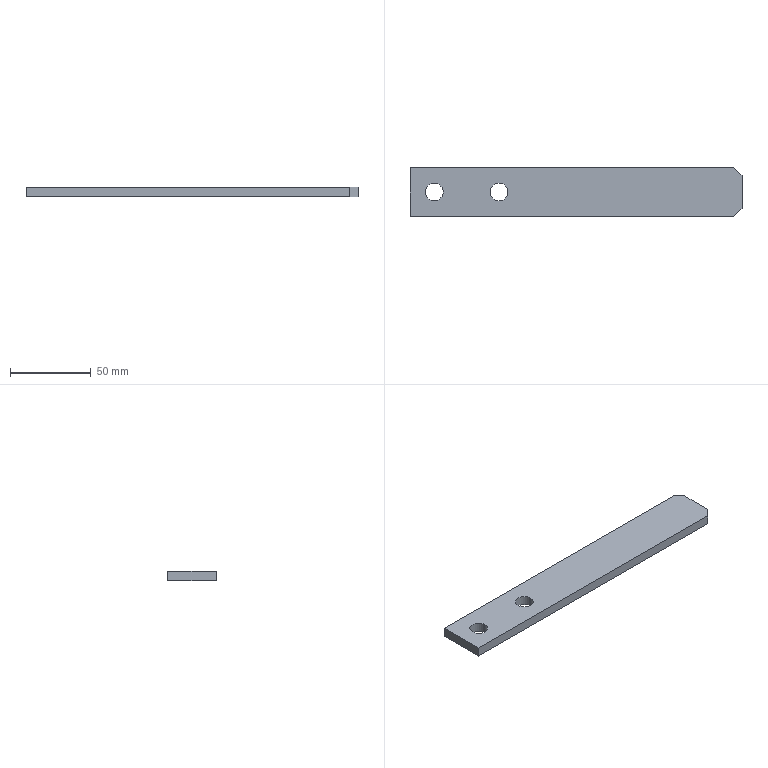Part | SolidWorks | features Extrusion 1 | 1 solid | 12 faces | box 205 x 30 x 6 mm | volume 35610 mm3 | plane 8 | cylinder 4 | commonest cylinder face diameters 11 x4
STEP:
#1=CARTESIAN_POINT('',(-53.,0.,-3.));
#2=VERTEX_POINT('',#1);
#3=CARTESIAN_POINT('',(-42.,0.,-3.));
#4=VERTEX_POINT('',#3);
#5=CARTESIAN_POINT('',(-47.5,0.,-3.));
#6=DIRECTION('',(0.,0.,1.));
#7=DIRECTION('',(-1.,0.,0.));
#8=AXIS2_PLACEMENT_3D('',#5,#6,#7);
#9=CIRCLE('',#8,5.5);
#10=EDGE_CURVE('',#2,#4,#9,.T.);
#11=ORIENTED_EDGE('',*,*,#10,.F.);
#12=CARTESIAN_POINT('',(-53.,0.,3.));
#13=VERTEX_POINT('',#12);
#14=CARTESIAN_POINT('',(-53.,0.,-3.));
#15=DIRECTION('',(0.,0.,1.));
#16=VECTOR('',#15,1000.);
#17=LINE('',#14,#16);
#18=EDGE_CURVE('',#2,#13,#17,.T.);
#19=ORIENTED_EDGE('',*,*,#18,.T.);
#20=CARTESIAN_POINT('',(-42.,0.,3.));
#21=VERTEX_POINT('',#20);
#22=CARTESIAN_POINT('',(-47.5,0.,3.));
#23=DIRECTION('',(0.,0.,1.));
#24=DIRECTION('',(-1.,0.,0.));
#25=AXIS2_PLACEMENT_3D('',#22,#23,#24);
#26=CIRCLE('',#25,5.5);
#27=EDGE_CURVE('',#13,#21,#26,.T.);
#28=ORIENTED_EDGE('',*,*,#27,.T.);
#29=CARTESIAN_POINT('',(-42.,0.,-3.));
#30=DIRECTION('',(0.,0.,1.));
#31=VECTOR('',#30,1000.);
#32=LINE('',#29,#31);
#33=EDGE_CURVE('',#4,#21,#32,.T.);
#34=ORIENTED_EDGE('',*,*,#33,.F.);
#35=EDGE_LOOP('',(#11,#19,#28,#34));
#36=FACE_OUTER_BOUND('',#35,.T.);
#37=CARTESIAN_POINT('',(-47.5,0.,-3.));
#38=DIRECTION('',(0.,0.,1.));
#39=DIRECTION('',(1.,0.,0.));
#40=AXIS2_PLACEMENT_3D('',#37,#38,#39);
#41=CYLINDRICAL_SURFACE('',#40,5.5);
#42=ADVANCED_FACE('',(#36),#41,.F.);
#43=CARTESIAN_POINT('',(-93.,0.,-3.));
#44=VERTEX_POINT('',#43);
#45=CARTESIAN_POINT('',(-82.,0.,-3.));
#46=VERTEX_POINT('',#45);
#47=CARTESIAN_POINT('',(-87.5,0.,-3.));
#48=DIRECTION('',(0.,0.,1.));
#49=DIRECTION('',(-1.,0.,0.));
#50=AXIS2_PLACEMENT_3D('',#47,#48,#49);
#51=CIRCLE('',#50,5.5);
#52=EDGE_CURVE('',#44,#46,#51,.T.);
#53=ORIENTED_EDGE('',*,*,#52,.F.);
#54=CARTESIAN_POINT('',(-93.,0.,3.));
#55=VERTEX_POINT('',#54);
#56=CARTESIAN_POINT('',(-93.,0.,-3.));
#57=DIRECTION('',(0.,0.,1.));
#58=VECTOR('',#57,1000.);
#59=LINE('',#56,#58);
#60=EDGE_CURVE('',#44,#55,#59,.T.);
#61=ORIENTED_EDGE('',*,*,#60,.T.);
#62=CARTESIAN_POINT('',(-82.,0.,3.));
#63=VERTEX_POINT('',#62);
#64=CARTESIAN_POINT('',(-87.5,0.,3.));
#65=DIRECTION('',(0.,0.,1.));
#66=DIRECTION('',(-1.,0.,0.));
#67=AXIS2_PLACEMENT_3D('',#64,#65,#66);
#68=CIRCLE('',#67,5.5);
#69=EDGE_CURVE('',#55,#63,#68,.T.);
#70=ORIENTED_EDGE('',*,*,#69,.T.);
#71=CARTESIAN_POINT('',(-82.,0.,-3.));
#72=DIRECTION('',(0.,0.,1.));
#73=VECTOR('',#72,1000.);
#74=LINE('',#71,#73);
#75=EDGE_CURVE('',#46,#63,#74,.T.);
#76=ORIENTED_EDGE('',*,*,#75,.F.);
#77=EDGE_LOOP('',(#53,#61,#70,#76));
#78=FACE_OUTER_BOUND('',#77,.T.);
#79=CARTESIAN_POINT('',(-87.5,0.,-3.));
#80=DIRECTION('',(0.,0.,1.));
#81=DIRECTION('',(1.,0.,0.));
#82=AXIS2_PLACEMENT_3D('',#79,#80,#81);
#83=CYLINDRICAL_SURFACE('',#82,5.5);
#84=ADVANCED_FACE('',(#78),#83,.F.);
#85=CARTESIAN_POINT('',(97.5,-15.,3.));
#86=VERTEX_POINT('',#85);
#87=CARTESIAN_POINT('',(102.5,-10.,3.));
#88=VERTEX_POINT('',#87);
#89=CARTESIAN_POINT('',(97.5,-15.,3.));
#90=DIRECTION('',(0.7071,0.7071,0.));
#91=VECTOR('',#90,1000.);
#92=LINE('',#89,#91);
#93=EDGE_CURVE('',#86,#88,#92,.T.);
#94=ORIENTED_EDGE('',*,*,#93,.F.);
#95=CARTESIAN_POINT('',(97.5,-15.,-3.));
#96=VERTEX_POINT('',#95);
#97=CARTESIAN_POINT('',(97.5,-15.,-3.));
#98=DIRECTION('',(0.,0.,1.));
#99=VECTOR('',#98,1000.);
#100=LINE('',#97,#99);
#101=EDGE_CURVE('',#96,#86,#100,.T.);
#102=ORIENTED_EDGE('',*,*,#101,.F.);
#103=CARTESIAN_POINT('',(102.5,-10.,-3.));
#104=VERTEX_POINT('',#103);
#105=CARTESIAN_POINT('',(97.5,-15.,-3.));
#106=DIRECTION('',(0.7071,0.7071,0.));
#107=VECTOR('',#106,1000.);
#108=LINE('',#105,#107);
#109=EDGE_CURVE('',#96,#104,#108,.T.);
#110=ORIENTED_EDGE('',*,*,#109,.T.);
#111=CARTESIAN_POINT('',(102.5,-10.,-3.));
#112=DIRECTION('',(0.,0.,1.));
#113=VECTOR('',#112,1000.);
#114=LINE('',#111,#113);
#115=EDGE_CURVE('',#104,#88,#114,.T.);
#116=ORIENTED_EDGE('',*,*,#115,.T.);
#117=EDGE_LOOP('',(#94,#102,#110,#116));
#118=FACE_OUTER_BOUND('',#117,.T.);
#119=CARTESIAN_POINT('',(97.5,-15.,-3.));
#120=DIRECTION('',(0.7071,-0.7071,0.));
#121=DIRECTION('',(0.7071,0.7071,0.));
#122=AXIS2_PLACEMENT_3D('',#119,#120,#121);
#123=PLANE('',#122);
#124=ADVANCED_FACE('',(#118),#123,.T.);
#125=CARTESIAN_POINT('',(-102.5,-15.,3.));
#126=VERTEX_POINT('',#125);
#127=CARTESIAN_POINT('',(-102.5,-15.,3.));
#128=DIRECTION('',(1.,0.,0.));
#129=VECTOR('',#128,1000.);
#130=LINE('',#127,#129);
#131=EDGE_CURVE('',#126,#86,#130,.T.);
#132=ORIENTED_EDGE('',*,*,#131,.F.);
#133=CARTESIAN_POINT('',(-102.5,-15.,-3.));
#134=VERTEX_POINT('',#133);
#135=CARTESIAN_POINT('',(-102.5,-15.,-3.));
#136=DIRECTION('',(0.,0.,1.));
#137=VECTOR('',#136,1000.);
#138=LINE('',#135,#137);
#139=EDGE_CURVE('',#134,#126,#138,.T.);
#140=ORIENTED_EDGE('',*,*,#139,.F.);
#141=CARTESIAN_POINT('',(-102.5,-15.,-3.));
#142=DIRECTION('',(1.,0.,0.));
#143=VECTOR('',#142,1000.);
#144=LINE('',#141,#143);
#145=EDGE_CURVE('',#134,#96,#144,.T.);
#146=ORIENTED_EDGE('',*,*,#145,.T.);
#147=ORIENTED_EDGE('',*,*,#101,.T.);
#148=EDGE_LOOP('',(#132,#140,#146,#147));
#149=FACE_OUTER_BOUND('',#148,.T.);
#150=CARTESIAN_POINT('',(-102.5,-15.,-3.));
#151=DIRECTION('',(0.,-1.,0.));
#152=DIRECTION('',(0.,0.,-1.));
#153=AXIS2_PLACEMENT_3D('',#150,#151,#152);
#154=PLANE('',#153);
#155=ADVANCED_FACE('',(#149),#154,.T.);
#156=CARTESIAN_POINT('',(-102.5,15.,3.));
#157=VERTEX_POINT('',#156);
#158=CARTESIAN_POINT('',(-102.5,15.,3.));
#159=DIRECTION('',(0.,-1.,0.));
#160=VECTOR('',#159,1000.);
#161=LINE('',#158,#160);
#162=EDGE_CURVE('',#157,#126,#161,.T.);
#163=ORIENTED_EDGE('',*,*,#162,.F.);
#164=CARTESIAN_POINT('',(-102.5,15.,-3.));
#165=VERTEX_POINT('',#164);
#166=CARTESIAN_POINT('',(-102.5,15.,-3.));
#167=DIRECTION('',(0.,0.,1.));
#168=VECTOR('',#167,1000.);
#169=LINE('',#166,#168);
#170=EDGE_CURVE('',#165,#157,#169,.T.);
#171=ORIENTED_EDGE('',*,*,#170,.F.);
#172=CARTESIAN_POINT('',(-102.5,15.,-3.));
#173=DIRECTION('',(0.,-1.,0.));
#174=VECTOR('',#173,1000.);
#175=LINE('',#172,#174);
#176=EDGE_CURVE('',#165,#134,#175,.T.);
#177=ORIENTED_EDGE('',*,*,#176,.T.);
#178=ORIENTED_EDGE('',*,*,#139,.T.);
#179=EDGE_LOOP('',(#163,#171,#177,#178));
#180=FACE_OUTER_BOUND('',#179,.T.);
#181=CARTESIAN_POINT('',(-102.5,15.,-3.));
#182=DIRECTION('',(-1.,0.,0.));
#183=DIRECTION('',(0.,0.,1.));
#184=AXIS2_PLACEMENT_3D('',#181,#182,#183);
#185=PLANE('',#184);
#186=ADVANCED_FACE('',(#180),#185,.T.);
#187=CARTESIAN_POINT('',(97.5,15.,3.));
#188=VERTEX_POINT('',#187);
#189=CARTESIAN_POINT('',(97.5,15.,3.));
#190=DIRECTION('',(-1.,0.,0.));
#191=VECTOR('',#190,1000.);
#192=LINE('',#189,#191);
#193=EDGE_CURVE('',#188,#157,#192,.T.);
#194=ORIENTED_EDGE('',*,*,#193,.F.);
#195=CARTESIAN_POINT('',(97.5,15.,-3.));
#196=VERTEX_POINT('',#195);
#197=CARTESIAN_POINT('',(97.5,15.,-3.));
#198=DIRECTION('',(0.,0.,1.));
#199=VECTOR('',#198,1000.);
#200=LINE('',#197,#199);
#201=EDGE_CURVE('',#196,#188,#200,.T.);
#202=ORIENTED_EDGE('',*,*,#201,.F.);
#203=CARTESIAN_POINT('',(97.5,15.,-3.));
#204=DIRECTION('',(-1.,0.,0.));
#205=VECTOR('',#204,1000.);
#206=LINE('',#203,#205);
#207=EDGE_CURVE('',#196,#165,#206,.T.);
#208=ORIENTED_EDGE('',*,*,#207,.T.);
#209=ORIENTED_EDGE('',*,*,#170,.T.);
#210=EDGE_LOOP('',(#194,#202,#208,#209));
#211=FACE_OUTER_BOUND('',#210,.T.);
#212=CARTESIAN_POINT('',(97.5,15.,-3.));
#213=DIRECTION('',(0.,1.,0.));
#214=DIRECTION('',(0.,0.,1.));
#215=AXIS2_PLACEMENT_3D('',#212,#213,#214);
#216=PLANE('',#215);
#217=ADVANCED_FACE('',(#211),#216,.T.);
#218=CARTESIAN_POINT('',(102.5,10.,3.));
#219=VERTEX_POINT('',#218);
#220=CARTESIAN_POINT('',(102.5,10.,3.));
#221=DIRECTION('',(-0.7071,0.7071,0.));
#222=VECTOR('',#221,1000.);
#223=LINE('',#220,#222);
#224=EDGE_CURVE('',#219,#188,#223,.T.);
#225=ORIENTED_EDGE('',*,*,#224,.F.);
#226=CARTESIAN_POINT('',(102.5,10.,-3.));
#227=VERTEX_POINT('',#226);
#228=CARTESIAN_POINT('',(102.5,10.,-3.));
#229=DIRECTION('',(0.,0.,1.));
#230=VECTOR('',#229,1000.);
#231=LINE('',#228,#230);
#232=EDGE_CURVE('',#227,#219,#231,.T.);
#233=ORIENTED_EDGE('',*,*,#232,.F.);
#234=CARTESIAN_POINT('',(102.5,10.,-3.));
#235=DIRECTION('',(-0.7071,0.7071,0.));
#236=VECTOR('',#235,1000.);
#237=LINE('',#234,#236);
#238=EDGE_CURVE('',#227,#196,#237,.T.);
#239=ORIENTED_EDGE('',*,*,#238,.T.);
#240=ORIENTED_EDGE('',*,*,#201,.T.);
#241=EDGE_LOOP('',(#225,#233,#239,#240));
#242=FACE_OUTER_BOUND('',#241,.T.);
#243=CARTESIAN_POINT('',(102.5,10.,-3.));
#244=DIRECTION('',(0.7071,0.7071,0.));
#245=DIRECTION('',(-0.7071,0.7071,0.));
#246=AXIS2_PLACEMENT_3D('',#243,#244,#245);
#247=PLANE('',#246);
#248=ADVANCED_FACE('',(#242),#247,.T.);
#249=CARTESIAN_POINT('',(102.5,-10.,3.));
#250=DIRECTION('',(0.,1.,0.));
#251=VECTOR('',#250,1000.);
#252=LINE('',#249,#251);
#253=EDGE_CURVE('',#88,#219,#252,.T.);
#254=ORIENTED_EDGE('',*,*,#253,.F.);
#255=ORIENTED_EDGE('',*,*,#115,.F.);
#256=CARTESIAN_POINT('',(102.5,-10.,-3.));
#257=DIRECTION('',(0.,1.,0.));
#258=VECTOR('',#257,1000.);
#259=LINE('',#256,#258);
#260=EDGE_CURVE('',#104,#227,#259,.T.);
#261=ORIENTED_EDGE('',*,*,#260,.T.);
#262=ORIENTED_EDGE('',*,*,#232,.T.);
#263=EDGE_LOOP('',(#254,#255,#261,#262));
#264=FACE_OUTER_BOUND('',#263,.T.);
#265=CARTESIAN_POINT('',(102.5,-10.,-3.));
#266=DIRECTION('',(1.,0.,0.));
#267=DIRECTION('',(0.,0.,-1.));
#268=AXIS2_PLACEMENT_3D('',#265,#266,#267);
#269=PLANE('',#268);
#270=ADVANCED_FACE('',(#264),#269,.T.);
#271=CARTESIAN_POINT('',(-47.5,0.,-3.));
#272=DIRECTION('',(0.,0.,1.));
#273=DIRECTION('',(-1.,0.,0.));
#274=AXIS2_PLACEMENT_3D('',#271,#272,#273);
#275=CIRCLE('',#274,5.5);
#276=EDGE_CURVE('',#4,#2,#275,.T.);
#277=ORIENTED_EDGE('',*,*,#276,.T.);
#278=ORIENTED_EDGE('',*,*,#10,.T.);
#279=EDGE_LOOP('',(#277,#278));
#280=FACE_BOUND('',#279,.T.);
#281=CARTESIAN_POINT('',(-87.5,0.,-3.));
#282=DIRECTION('',(0.,0.,1.));
#283=DIRECTION('',(-1.,0.,0.));
#284=AXIS2_PLACEMENT_3D('',#281,#282,#283);
#285=CIRCLE('',#284,5.5);
#286=EDGE_CURVE('',#46,#44,#285,.T.);
#287=ORIENTED_EDGE('',*,*,#286,.T.);
#288=ORIENTED_EDGE('',*,*,#52,.T.);
#289=EDGE_LOOP('',(#287,#288));
#290=FACE_BOUND('',#289,.T.);
#291=ORIENTED_EDGE('',*,*,#109,.F.);
#292=ORIENTED_EDGE('',*,*,#145,.F.);
#293=ORIENTED_EDGE('',*,*,#176,.F.);
#294=ORIENTED_EDGE('',*,*,#207,.F.);
#295=ORIENTED_EDGE('',*,*,#238,.F.);
#296=ORIENTED_EDGE('',*,*,#260,.F.);
#297=EDGE_LOOP('',(#291,#292,#293,#294,#295,#296));
#298=FACE_OUTER_BOUND('',#297,.T.);
#299=CARTESIAN_POINT('',(0.,0.,-3.));
#300=DIRECTION('',(0.,0.,1.));
#301=DIRECTION('',(1.,0.,0.));
#302=AXIS2_PLACEMENT_3D('',#299,#300,#301);
#303=PLANE('',#302);
#304=ADVANCED_FACE('',(#280,#290,#298),#303,.F.);
#305=CARTESIAN_POINT('',(-47.5,0.,3.));
#306=DIRECTION('',(0.,0.,1.));
#307=DIRECTION('',(-1.,0.,0.));
#308=AXIS2_PLACEMENT_3D('',#305,#306,#307);
#309=CIRCLE('',#308,5.5);
#310=EDGE_CURVE('',#21,#13,#309,.T.);
#311=ORIENTED_EDGE('',*,*,#310,.F.);
#312=ORIENTED_EDGE('',*,*,#27,.F.);
#313=EDGE_LOOP('',(#311,#312));
#314=FACE_BOUND('',#313,.T.);
#315=CARTESIAN_POINT('',(-87.5,0.,3.));
#316=DIRECTION('',(0.,0.,1.));
#317=DIRECTION('',(-1.,0.,0.));
#318=AXIS2_PLACEMENT_3D('',#315,#316,#317);
#319=CIRCLE('',#318,5.5);
#320=EDGE_CURVE('',#63,#55,#319,.T.);
#321=ORIENTED_EDGE('',*,*,#320,.F.);
#322=ORIENTED_EDGE('',*,*,#69,.F.);
#323=EDGE_LOOP('',(#321,#322));
#324=FACE_BOUND('',#323,.T.);
#325=ORIENTED_EDGE('',*,*,#93,.T.);
#326=ORIENTED_EDGE('',*,*,#253,.T.);
#327=ORIENTED_EDGE('',*,*,#224,.T.);
#328=ORIENTED_EDGE('',*,*,#193,.T.);
#329=ORIENTED_EDGE('',*,*,#162,.T.);
#330=ORIENTED_EDGE('',*,*,#131,.T.);
#331=EDGE_LOOP('',(#325,#326,#327,#328,#329,#330));
#332=FACE_OUTER_BOUND('',#331,.T.);
#333=CARTESIAN_POINT('',(0.,0.,3.));
#334=DIRECTION('',(0.,0.,1.));
#335=DIRECTION('',(1.,0.,0.));
#336=AXIS2_PLACEMENT_3D('',#333,#334,#335);
#337=PLANE('',#336);
#338=ADVANCED_FACE('',(#314,#324,#332),#337,.T.);
#339=ORIENTED_EDGE('',*,*,#60,.F.);
#340=ORIENTED_EDGE('',*,*,#286,.F.);
#341=ORIENTED_EDGE('',*,*,#75,.T.);
#342=ORIENTED_EDGE('',*,*,#320,.T.);
#343=EDGE_LOOP('',(#339,#340,#341,#342));
#344=FACE_OUTER_BOUND('',#343,.T.);
#345=CARTESIAN_POINT('',(-87.5,0.,-3.));
#346=DIRECTION('',(0.,0.,1.));
#347=DIRECTION('',(1.,0.,0.));
#348=AXIS2_PLACEMENT_3D('',#345,#346,#347);
#349=CYLINDRICAL_SURFACE('',#348,5.5);
#350=ADVANCED_FACE('',(#344),#349,.F.);
#351=ORIENTED_EDGE('',*,*,#18,.F.);
#352=ORIENTED_EDGE('',*,*,#276,.F.);
#353=ORIENTED_EDGE('',*,*,#33,.T.);
#354=ORIENTED_EDGE('',*,*,#310,.T.);
#355=EDGE_LOOP('',(#351,#352,#353,#354));
#356=FACE_OUTER_BOUND('',#355,.T.);
#357=CARTESIAN_POINT('',(-47.5,0.,-3.));
#358=DIRECTION('',(0.,0.,1.));
#359=DIRECTION('',(1.,0.,0.));
#360=AXIS2_PLACEMENT_3D('',#357,#358,#359);
#361=CYLINDRICAL_SURFACE('',#360,5.5);
#362=ADVANCED_FACE('',(#356),#361,.F.);
#363=CLOSED_SHELL('',(#42,#84,#124,#155,#186,#217,#248,#270,#304,#338,#350,#362));
#364=MANIFOLD_SOLID_BREP('',#363);
#365=CARTESIAN_POINT('',(0.,0.,0.));
#366=DIRECTION('',(0.,0.,1.));
#367=DIRECTION('',(1.,0.,0.));
#368=AXIS2_PLACEMENT_3D('',#365,#366,#367);
#369=(LENGTH_UNIT()NAMED_UNIT(*)SI_UNIT(.MILLI.,.METRE.));
#370=UNCERTAINTY_MEASURE_WITH_UNIT(LENGTH_MEASURE(0.00001),#369,'','');
#371=(NAMED_UNIT(*)PLANE_ANGLE_UNIT()SI_UNIT($,.RADIAN.));
#372=(NAMED_UNIT(*)SI_UNIT($,.STERADIAN.)SOLID_ANGLE_UNIT());
#373=(GEOMETRIC_REPRESENTATION_CONTEXT(3)GLOBAL_UNCERTAINTY_ASSIGNED_CONTEXT((#370))GLOBAL_UNIT_ASSIGNED_CONTEXT((#369,#371,#372))REPRESENTATION_CONTEXT('',''));
#374=ADVANCED_BREP_SHAPE_REPRESENTATION('',(#364,#368),#373);